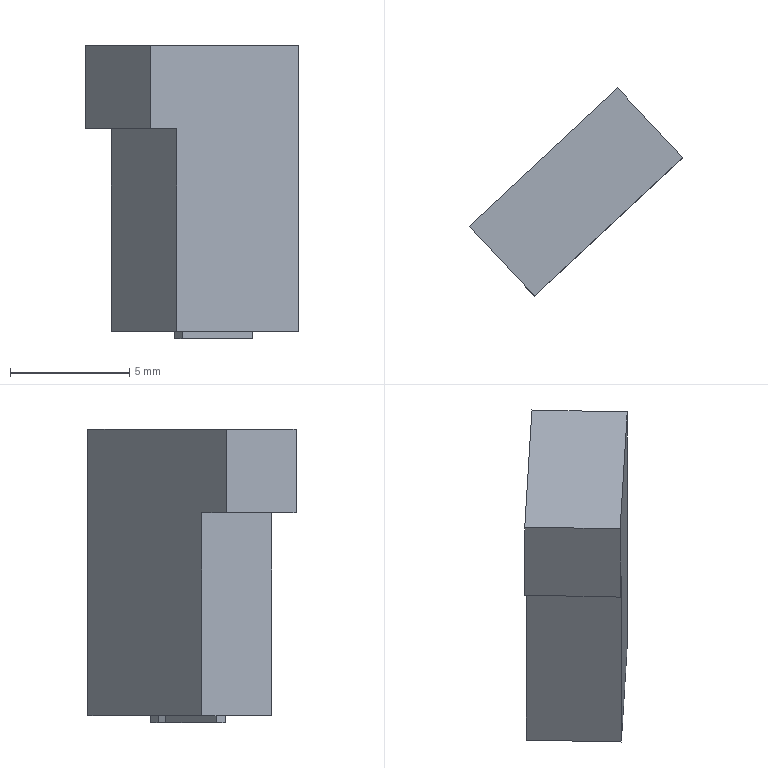Part | STEP file | gslz 2016.10.28-13_id950_x_t | 1 solid | 16 faces | box 8.945 x 8.722 x 12.3 mm | volume 357.729 mm3 | plane 15 | cylinder 1 | commonest cylinder face diameters 5.012 x1
STEP:
#1=CARTESIAN_POINT('',(0.,0.,0.));
#2=DIRECTION('',(0.,0.,1.));
#3=DIRECTION('',(1.,0.,0.));
#4=AXIS2_PLACEMENT_3D('',#1,#2,#3);
#5=CARTESIAN_POINT('',(-462.885,146.364,1.25));
#6=VERTEX_POINT('',#5);
#7=CARTESIAN_POINT('',(-462.538,146.688,1.25));
#8=VERTEX_POINT('',#7);
#9=CARTESIAN_POINT('',(-462.885,146.364,1.25));
#10=DIRECTION('',(0.7314,0.682,0.));
#11=VECTOR('',#10,1.);
#12=LINE('',#9,#11);
#13=CARTESIAN_POINT('',(-464.11,157.886,1.25));
#14=DIRECTION('',(0.,0.,-1.));
#15=DIRECTION('',(0.7314,0.682,0.));
#16=AXIS2_PLACEMENT_3D('',#13,#14,#15);
#17=PLANE('',#16);
#18=CARTESIAN_POINT('',(-6.962,9.262));
#19=DIRECTION('',(1.,0.));
#20=VECTOR('',#19,1.);
#21=LINE('',#18,#20);
#22=(GEOMETRIC_REPRESENTATION_CONTEXT(2)PARAMETRIC_REPRESENTATION_CONTEXT()REPRESENTATION_CONTEXT('',''));
#23=DEFINITIONAL_REPRESENTATION('',(#21),#22);
#24=PCURVE('',#17,#23);
#25=CARTESIAN_POINT('',(-462.885,146.364,0.95));
#26=DIRECTION('',(0.682,-0.7314,0.));
#27=DIRECTION('',(0.,0.,-1.));
#28=AXIS2_PLACEMENT_3D('',#25,#26,#27);
#29=PLANE('',#28);
#30=CARTESIAN_POINT('',(-0.3,0.));
#31=DIRECTION('',(0.,1.));
#32=VECTOR('',#31,1.);
#33=LINE('',#30,#32);
#34=(GEOMETRIC_REPRESENTATION_CONTEXT(2)PARAMETRIC_REPRESENTATION_CONTEXT()REPRESENTATION_CONTEXT('',''));
#35=DEFINITIONAL_REPRESENTATION('',(#33),#34);
#36=PCURVE('',#29,#35);
#37=SURFACE_CURVE('',#12,(#24,#36),.PCURVE_S1.);
#38=EDGE_CURVE('',#6,#8,#37,.T.);
#39=ORIENTED_EDGE('',*,*,#38,.F.);
#40=CARTESIAN_POINT('',(-461.783,146.049,1.25));
#41=VERTEX_POINT('',#40);
#42=CARTESIAN_POINT('',(-461.783,146.049,1.25));
#43=DIRECTION('',(-0.9615,0.2748,0.));
#44=VECTOR('',#43,1.);
#45=LINE('',#42,#44);
#46=CARTESIAN_POINT('',(-6.371,10.245));
#47=DIRECTION('',(-0.5158,-0.8567));
#48=VECTOR('',#47,1.);
#49=LINE('',#46,#48);
#50=(GEOMETRIC_REPRESENTATION_CONTEXT(2)PARAMETRIC_REPRESENTATION_CONTEXT()REPRESENTATION_CONTEXT('',''));
#51=DEFINITIONAL_REPRESENTATION('',(#49),#50);
#52=PCURVE('',#17,#51);
#53=CARTESIAN_POINT('',(-461.783,146.049,0.95));
#54=DIRECTION('',(0.2748,0.9615,0.));
#55=DIRECTION('',(-0.9615,0.2748,0.));
#56=AXIS2_PLACEMENT_3D('',#53,#54,#55);
#57=PLANE('',#56);
#58=CARTESIAN_POINT('',(0.,0.3));
#59=DIRECTION('',(1.,0.));
#60=VECTOR('',#59,1.);
#61=LINE('',#58,#60);
#62=(GEOMETRIC_REPRESENTATION_CONTEXT(2)PARAMETRIC_REPRESENTATION_CONTEXT()REPRESENTATION_CONTEXT('',''));
#63=DEFINITIONAL_REPRESENTATION('',(#61),#62);
#64=PCURVE('',#57,#63);
#65=SURFACE_CURVE('',#45,(#52,#64),.PCURVE_S1.);
#66=EDGE_CURVE('',#41,#6,#65,.T.);
#67=ORIENTED_EDGE('',*,*,#66,.F.);
#68=CARTESIAN_POINT('',(-464.072,143.915,1.25));
#69=VERTEX_POINT('',#68);
#70=CARTESIAN_POINT('',(-464.072,143.915,1.25));
#71=DIRECTION('',(0.7314,0.682,0.));
#72=VECTOR('',#71,1.);
#73=LINE('',#70,#72);
#74=CARTESIAN_POINT('',(-9.5,10.245));
#75=DIRECTION('',(1.,0.));
#76=VECTOR('',#75,1.);
#77=LINE('',#74,#76);
#78=(GEOMETRIC_REPRESENTATION_CONTEXT(2)PARAMETRIC_REPRESENTATION_CONTEXT()REPRESENTATION_CONTEXT('',''));
#79=DEFINITIONAL_REPRESENTATION('',(#77),#78);
#80=PCURVE('',#17,#79);
#81=CARTESIAN_POINT('',(-464.072,143.915,0.95));
#82=DIRECTION('',(0.682,-0.7314,0.));
#83=DIRECTION('',(0.,0.,-1.));
#84=AXIS2_PLACEMENT_3D('',#81,#82,#83);
#85=PLANE('',#84);
#86=CARTESIAN_POINT('',(-0.3,0.));
#87=DIRECTION('',(0.,1.));
#88=VECTOR('',#87,1.);
#89=LINE('',#86,#88);
#90=(GEOMETRIC_REPRESENTATION_CONTEXT(2)PARAMETRIC_REPRESENTATION_CONTEXT()REPRESENTATION_CONTEXT('',''));
#91=DEFINITIONAL_REPRESENTATION('',(#89),#90);
#92=PCURVE('',#85,#91);
#93=SURFACE_CURVE('',#73,(#80,#92),.PCURVE_S1.);
#94=EDGE_CURVE('',#69,#41,#93,.T.);
#95=ORIENTED_EDGE('',*,*,#94,.F.);
#96=CARTESIAN_POINT('',(-463.737,143.555,1.25));
#97=VERTEX_POINT('',#96);
#98=CARTESIAN_POINT('',(-463.737,143.555,1.25));
#99=DIRECTION('',(-0.682,0.7314,0.));
#100=VECTOR('',#99,1.);
#101=LINE('',#98,#100);
#102=CARTESIAN_POINT('',(-9.5,10.736));
#103=DIRECTION('',(0.,-1.));
#104=VECTOR('',#103,1.);
#105=LINE('',#102,#104);
#106=(GEOMETRIC_REPRESENTATION_CONTEXT(2)PARAMETRIC_REPRESENTATION_CONTEXT()REPRESENTATION_CONTEXT('',''));
#107=DEFINITIONAL_REPRESENTATION('',(#105),#106);
#108=PCURVE('',#17,#107);
#109=CARTESIAN_POINT('',(-463.737,143.555,0.95));
#110=DIRECTION('',(0.7314,0.682,0.));
#111=DIRECTION('',(0.,0.,1.));
#112=AXIS2_PLACEMENT_3D('',#109,#110,#111);
#113=PLANE('',#112);
#114=CARTESIAN_POINT('',(0.3,0.));
#115=DIRECTION('',(0.,-1.));
#116=VECTOR('',#115,1.);
#117=LINE('',#114,#116);
#118=(GEOMETRIC_REPRESENTATION_CONTEXT(2)PARAMETRIC_REPRESENTATION_CONTEXT()REPRESENTATION_CONTEXT('',''));
#119=DEFINITIONAL_REPRESENTATION('',(#117),#118);
#120=PCURVE('',#113,#119);
#121=SURFACE_CURVE('',#101,(#108,#120),.PCURVE_S1.);
#122=EDGE_CURVE('',#97,#69,#121,.T.);
#123=ORIENTED_EDGE('',*,*,#122,.F.);
#124=CARTESIAN_POINT('',(-460.799,146.295,1.25));
#125=VERTEX_POINT('',#124);
#126=CARTESIAN_POINT('',(-460.799,146.295,1.25));
#127=DIRECTION('',(-0.7314,-0.682,0.));
#128=VECTOR('',#127,1.);
#129=LINE('',#126,#128);
#130=CARTESIAN_POINT('',(-5.484,10.736));
#131=DIRECTION('',(-1.,0.));
#132=VECTOR('',#131,1.);
#133=LINE('',#130,#132);
#134=(GEOMETRIC_REPRESENTATION_CONTEXT(2)PARAMETRIC_REPRESENTATION_CONTEXT()REPRESENTATION_CONTEXT('',''));
#135=DEFINITIONAL_REPRESENTATION('',(#133),#134);
#136=PCURVE('',#17,#135);
#137=CARTESIAN_POINT('',(-460.799,146.295,0.95));
#138=DIRECTION('',(-0.682,0.7314,0.));
#139=DIRECTION('',(0.,0.,1.));
#140=AXIS2_PLACEMENT_3D('',#137,#138,#139);
#141=PLANE('',#140);
#142=CARTESIAN_POINT('',(0.3,0.));
#143=DIRECTION('',(0.,-1.));
#144=VECTOR('',#143,1.);
#145=LINE('',#142,#144);
#146=(GEOMETRIC_REPRESENTATION_CONTEXT(2)PARAMETRIC_REPRESENTATION_CONTEXT()REPRESENTATION_CONTEXT('',''));
#147=DEFINITIONAL_REPRESENTATION('',(#145),#146);
#148=PCURVE('',#141,#147);
#149=SURFACE_CURVE('',#129,(#136,#148),.PCURVE_S1.);
#150=EDGE_CURVE('',#125,#97,#149,.T.);
#151=ORIENTED_EDGE('',*,*,#150,.F.);
#152=CARTESIAN_POINT('',(-461.015,146.527,1.25));
#153=VERTEX_POINT('',#152);
#154=CARTESIAN_POINT('',(-461.015,146.527,1.25));
#155=DIRECTION('',(0.682,-0.7314,0.));
#156=VECTOR('',#155,1.);
#157=LINE('',#154,#156);
#158=CARTESIAN_POINT('',(-5.484,10.419));
#159=DIRECTION('',(0.,1.));
#160=VECTOR('',#159,1.);
#161=LINE('',#158,#160);
#162=(GEOMETRIC_REPRESENTATION_CONTEXT(2)PARAMETRIC_REPRESENTATION_CONTEXT()REPRESENTATION_CONTEXT('',''));
#163=DEFINITIONAL_REPRESENTATION('',(#161),#162);
#164=PCURVE('',#17,#163);
#165=CARTESIAN_POINT('',(-461.015,146.527,0.95));
#166=DIRECTION('',(-0.7314,-0.682,0.));
#167=DIRECTION('',(0.,0.,-1.));
#168=AXIS2_PLACEMENT_3D('',#165,#166,#167);
#169=PLANE('',#168);
#170=CARTESIAN_POINT('',(-0.3,0.));
#171=DIRECTION('',(0.,1.));
#172=VECTOR('',#171,1.);
#173=LINE('',#170,#172);
#174=(GEOMETRIC_REPRESENTATION_CONTEXT(2)PARAMETRIC_REPRESENTATION_CONTEXT()REPRESENTATION_CONTEXT('',''));
#175=DEFINITIONAL_REPRESENTATION('',(#173),#174);
#176=PCURVE('',#169,#175);
#177=SURFACE_CURVE('',#157,(#164,#176),.PCURVE_S1.);
#178=EDGE_CURVE('',#153,#125,#177,.T.);
#179=ORIENTED_EDGE('',*,*,#178,.F.);
#180=CARTESIAN_POINT('',(-461.526,148.98,1.25));
#181=DIRECTION('',(0.,0.,1.));
#182=DIRECTION('',(0.682,-0.7314,0.));
#183=AXIS2_PLACEMENT_3D('',#180,#181,#182);
#184=CIRCLE('',#183,2.506);
#185=CARTESIAN_POINT('',(-4.184,10.782));
#186=CARTESIAN_POINT('',(0.1568,10.782));
#187=CARTESIAN_POINT('',(-2.013,7.023));
#188=CARTESIAN_POINT('',(-4.184,3.264));
#189=CARTESIAN_POINT('',(-6.354,7.023));
#190=CARTESIAN_POINT('',(-8.524,10.782));
#191=CARTESIAN_POINT('',(-4.184,10.782));
#192=(BOUNDED_CURVE()B_SPLINE_CURVE(2,(#185,#186,#187,#188,#189,#190,#191),.UNSPECIFIED.,.T.,.F.)B_SPLINE_CURVE_WITH_KNOTS((1,2,2,2,2,1),(-2.094,0.,2.094,4.189,6.283,8.378),.UNSPECIFIED.)CURVE()GEOMETRIC_REPRESENTATION_ITEM()RATIONAL_B_SPLINE_CURVE((1.,0.5,1.,0.5,1.,0.5,1.))REPRESENTATION_ITEM(''));
#193=(GEOMETRIC_REPRESENTATION_CONTEXT(2)PARAMETRIC_REPRESENTATION_CONTEXT()REPRESENTATION_CONTEXT('',''));
#194=DEFINITIONAL_REPRESENTATION('',(#192),#193);
#195=PCURVE('',#17,#194);
#196=CARTESIAN_POINT('',(-461.526,148.98,0.95));
#197=DIRECTION('',(0.,0.,1.));
#198=DIRECTION('',(0.682,-0.7314,0.));
#199=AXIS2_PLACEMENT_3D('',#196,#197,#198);
#200=CYLINDRICAL_SURFACE('',#199,2.506);
#201=CARTESIAN_POINT('',(0.,0.3));
#202=DIRECTION('',(1.,0.));
#203=VECTOR('',#202,1.);
#204=LINE('',#201,#203);
#205=(GEOMETRIC_REPRESENTATION_CONTEXT(2)PARAMETRIC_REPRESENTATION_CONTEXT()REPRESENTATION_CONTEXT('',''));
#206=DEFINITIONAL_REPRESENTATION('',(#204),#205);
#207=PCURVE('',#200,#206);
#208=SURFACE_CURVE('',#184,(#195,#207),.PCURVE_S1.);
#209=EDGE_CURVE('',#8,#153,#208,.T.);
#210=ORIENTED_EDGE('',*,*,#209,.F.);
#211=EDGE_LOOP('',(#39,#67,#95,#123,#151,#179,#210));
#212=FACE_BOUND('',#211,.T.);
#213=CARTESIAN_POINT('',(-466.7,144.534,1.25));
#214=VERTEX_POINT('',#213);
#215=CARTESIAN_POINT('',(-461.58,149.308,1.25));
#216=VERTEX_POINT('',#215);
#217=CARTESIAN_POINT('',(-466.7,144.534,1.25));
#218=DIRECTION('',(0.7314,0.682,0.));
#219=VECTOR('',#218,1.);
#220=LINE('',#217,#219);
#221=CARTESIAN_POINT('',(-11.,7.999));
#222=DIRECTION('',(1.,0.));
#223=VECTOR('',#222,1.);
#224=LINE('',#221,#223);
#225=(GEOMETRIC_REPRESENTATION_CONTEXT(2)PARAMETRIC_REPRESENTATION_CONTEXT()REPRESENTATION_CONTEXT('',''));
#226=DEFINITIONAL_REPRESENTATION('',(#224),#225);
#227=PCURVE('',#17,#226);
#228=CARTESIAN_POINT('',(-466.7,144.534,-0.75));
#229=DIRECTION('',(0.682,-0.7314,0.));
#230=DIRECTION('',(0.,0.,-1.));
#231=AXIS2_PLACEMENT_3D('',#228,#229,#230);
#232=PLANE('',#231);
#233=CARTESIAN_POINT('',(-2.,0.));
#234=DIRECTION('',(0.,1.));
#235=VECTOR('',#234,1.);
#236=LINE('',#233,#235);
#237=(GEOMETRIC_REPRESENTATION_CONTEXT(2)PARAMETRIC_REPRESENTATION_CONTEXT()REPRESENTATION_CONTEXT('',''));
#238=DEFINITIONAL_REPRESENTATION('',(#236),#237);
#239=PCURVE('',#232,#238);
#240=SURFACE_CURVE('',#220,(#227,#239),.PCURVE_S1.);
#241=EDGE_CURVE('',#214,#216,#240,.T.);
#242=ORIENTED_EDGE('',*,*,#241,.T.);
#243=CARTESIAN_POINT('',(-458.853,146.382,1.25));
#244=VERTEX_POINT('',#243);
#245=CARTESIAN_POINT('',(-461.58,149.308,1.25));
#246=DIRECTION('',(0.682,-0.7314,0.));
#247=VECTOR('',#246,1.);
#248=LINE('',#245,#247);
#249=CARTESIAN_POINT('',(-4.,7.999));
#250=DIRECTION('',(0.,1.));
#251=VECTOR('',#250,1.);
#252=LINE('',#249,#251);
#253=(GEOMETRIC_REPRESENTATION_CONTEXT(2)PARAMETRIC_REPRESENTATION_CONTEXT()REPRESENTATION_CONTEXT('',''));
#254=DEFINITIONAL_REPRESENTATION('',(#252),#253);
#255=PCURVE('',#17,#254);
#256=CARTESIAN_POINT('',(-461.58,149.308,-0.75));
#257=DIRECTION('',(-0.7314,-0.682,0.));
#258=DIRECTION('',(0.,0.,-1.));
#259=AXIS2_PLACEMENT_3D('',#256,#257,#258);
#260=PLANE('',#259);
#261=CARTESIAN_POINT('',(-2.,0.));
#262=DIRECTION('',(0.,1.));
#263=VECTOR('',#262,1.);
#264=LINE('',#261,#263);
#265=(GEOMETRIC_REPRESENTATION_CONTEXT(2)PARAMETRIC_REPRESENTATION_CONTEXT()REPRESENTATION_CONTEXT('',''));
#266=DEFINITIONAL_REPRESENTATION('',(#264),#265);
#267=PCURVE('',#260,#266);
#268=SURFACE_CURVE('',#248,(#255,#267),.PCURVE_S1.);
#269=EDGE_CURVE('',#216,#244,#268,.T.);
#270=ORIENTED_EDGE('',*,*,#269,.T.);
#271=CARTESIAN_POINT('',(-463.972,141.609,1.25));
#272=VERTEX_POINT('',#271);
#273=CARTESIAN_POINT('',(-458.853,146.382,1.25));
#274=DIRECTION('',(-0.7314,-0.682,0.));
#275=VECTOR('',#274,1.);
#276=LINE('',#273,#275);
#277=CARTESIAN_POINT('',(-4.,11.999));
#278=DIRECTION('',(-1.,0.));
#279=VECTOR('',#278,1.);
#280=LINE('',#277,#279);
#281=(GEOMETRIC_REPRESENTATION_CONTEXT(2)PARAMETRIC_REPRESENTATION_CONTEXT()REPRESENTATION_CONTEXT('',''));
#282=DEFINITIONAL_REPRESENTATION('',(#280),#281);
#283=PCURVE('',#17,#282);
#284=CARTESIAN_POINT('',(-458.853,146.382,-0.75));
#285=DIRECTION('',(-0.682,0.7314,0.));
#286=DIRECTION('',(0.,0.,1.));
#287=AXIS2_PLACEMENT_3D('',#284,#285,#286);
#288=PLANE('',#287);
#289=CARTESIAN_POINT('',(2.,0.));
#290=DIRECTION('',(0.,-1.));
#291=VECTOR('',#290,1.);
#292=LINE('',#289,#291);
#293=(GEOMETRIC_REPRESENTATION_CONTEXT(2)PARAMETRIC_REPRESENTATION_CONTEXT()REPRESENTATION_CONTEXT('',''));
#294=DEFINITIONAL_REPRESENTATION('',(#292),#293);
#295=PCURVE('',#288,#294);
#296=SURFACE_CURVE('',#276,(#283,#295),.PCURVE_S1.);
#297=EDGE_CURVE('',#244,#272,#296,.T.);
#298=ORIENTED_EDGE('',*,*,#297,.T.);
#299=CARTESIAN_POINT('',(-463.972,141.609,1.25));
#300=DIRECTION('',(-0.682,0.7314,0.));
#301=VECTOR('',#300,1.);
#302=LINE('',#299,#301);
#303=CARTESIAN_POINT('',(-11.,11.999));
#304=DIRECTION('',(0.,-1.));
#305=VECTOR('',#304,1.);
#306=LINE('',#303,#305);
#307=(GEOMETRIC_REPRESENTATION_CONTEXT(2)PARAMETRIC_REPRESENTATION_CONTEXT()REPRESENTATION_CONTEXT('',''));
#308=DEFINITIONAL_REPRESENTATION('',(#306),#307);
#309=PCURVE('',#17,#308);
#310=CARTESIAN_POINT('',(-463.972,141.609,-0.75));
#311=DIRECTION('',(0.7314,0.682,0.));
#312=DIRECTION('',(0.,0.,1.));
#313=AXIS2_PLACEMENT_3D('',#310,#311,#312);
#314=PLANE('',#313);
#315=CARTESIAN_POINT('',(2.,0.));
#316=DIRECTION('',(0.,-1.));
#317=VECTOR('',#316,1.);
#318=LINE('',#315,#317);
#319=(GEOMETRIC_REPRESENTATION_CONTEXT(2)PARAMETRIC_REPRESENTATION_CONTEXT()REPRESENTATION_CONTEXT('',''));
#320=DEFINITIONAL_REPRESENTATION('',(#318),#319);
#321=PCURVE('',#314,#320);
#322=SURFACE_CURVE('',#302,(#309,#321),.PCURVE_S1.);
#323=EDGE_CURVE('',#272,#214,#322,.T.);
#324=ORIENTED_EDGE('',*,*,#323,.T.);
#325=EDGE_LOOP('',(#242,#270,#298,#324));
#326=FACE_BOUND('',#325,.T.);
#327=ADVANCED_FACE('',(#212,#326),#17,.T.);
#328=CARTESIAN_POINT('',(-467.797,143.511,13.25));
#329=VERTEX_POINT('',#328);
#330=CARTESIAN_POINT('',(-461.58,149.308,13.25));
#331=VERTEX_POINT('',#330);
#332=CARTESIAN_POINT('',(-466.7,144.534,13.25));
#333=DIRECTION('',(0.7314,0.682,0.));
#334=VECTOR('',#333,1.);
#335=LINE('',#332,#334);
#336=CARTESIAN_POINT('',(-14.,0.));
#337=DIRECTION('',(0.,1.));
#338=VECTOR('',#337,1.);
#339=LINE('',#336,#338);
#340=(GEOMETRIC_REPRESENTATION_CONTEXT(2)PARAMETRIC_REPRESENTATION_CONTEXT()REPRESENTATION_CONTEXT('',''));
#341=DEFINITIONAL_REPRESENTATION('',(#339),#340);
#342=PCURVE('',#232,#341);
#343=CARTESIAN_POINT('',(-464.11,157.886,13.25));
#344=DIRECTION('',(0.,0.,-1.));
#345=DIRECTION('',(0.7314,0.682,0.));
#346=AXIS2_PLACEMENT_3D('',#343,#344,#345);
#347=PLANE('',#346);
#348=CARTESIAN_POINT('',(-11.,7.999));
#349=DIRECTION('',(1.,0.));
#350=VECTOR('',#349,1.);
#351=LINE('',#348,#350);
#352=(GEOMETRIC_REPRESENTATION_CONTEXT(2)PARAMETRIC_REPRESENTATION_CONTEXT()REPRESENTATION_CONTEXT('',''));
#353=DEFINITIONAL_REPRESENTATION('',(#351),#352);
#354=PCURVE('',#347,#353);
#355=SURFACE_CURVE('',#335,(#342,#354),.PCURVE_S1.);
#356=EDGE_CURVE('',#329,#331,#355,.T.);
#357=ORIENTED_EDGE('',*,*,#356,.T.);
#358=CARTESIAN_POINT('',(-461.58,149.308,-0.75));
#359=DIRECTION('',(0.,0.,1.));
#360=VECTOR('',#359,1.);
#361=LINE('',#358,#360);
#362=CARTESIAN_POINT('',(0.,7.));
#363=DIRECTION('',(-1.,0.));
#364=VECTOR('',#363,1.);
#365=LINE('',#362,#364);
#366=(GEOMETRIC_REPRESENTATION_CONTEXT(2)PARAMETRIC_REPRESENTATION_CONTEXT()REPRESENTATION_CONTEXT('',''));
#367=DEFINITIONAL_REPRESENTATION('',(#365),#366);
#368=PCURVE('',#232,#367);
#369=CARTESIAN_POINT('',(0.,0.));
#370=DIRECTION('',(-1.,0.));
#371=VECTOR('',#370,1.);
#372=LINE('',#369,#371);
#373=(GEOMETRIC_REPRESENTATION_CONTEXT(2)PARAMETRIC_REPRESENTATION_CONTEXT()REPRESENTATION_CONTEXT('',''));
#374=DEFINITIONAL_REPRESENTATION('',(#372),#373);
#375=PCURVE('',#260,#374);
#376=SURFACE_CURVE('',#361,(#368,#375),.PCURVE_S1.);
#377=EDGE_CURVE('',#216,#331,#376,.T.);
#378=ORIENTED_EDGE('',*,*,#377,.F.);
#379=ORIENTED_EDGE('',*,*,#241,.F.);
#380=CARTESIAN_POINT('',(-466.7,144.534,9.75));
#381=VERTEX_POINT('',#380);
#382=CARTESIAN_POINT('',(-466.7,144.534,-0.75));
#383=DIRECTION('',(0.,0.,1.));
#384=VECTOR('',#383,1.);
#385=LINE('',#382,#384);
#386=CARTESIAN_POINT('',(0.,0.));
#387=DIRECTION('',(-1.,0.));
#388=VECTOR('',#387,1.);
#389=LINE('',#386,#388);
#390=(GEOMETRIC_REPRESENTATION_CONTEXT(2)PARAMETRIC_REPRESENTATION_CONTEXT()REPRESENTATION_CONTEXT('',''));
#391=DEFINITIONAL_REPRESENTATION('',(#389),#390);
#392=PCURVE('',#232,#391);
#393=CARTESIAN_POINT('',(0.,-4.));
#394=DIRECTION('',(1.,0.));
#395=VECTOR('',#394,1.);
#396=LINE('',#393,#395);
#397=(GEOMETRIC_REPRESENTATION_CONTEXT(2)PARAMETRIC_REPRESENTATION_CONTEXT()REPRESENTATION_CONTEXT('',''));
#398=DEFINITIONAL_REPRESENTATION('',(#396),#397);
#399=PCURVE('',#314,#398);
#400=SURFACE_CURVE('',#385,(#392,#399),.PCURVE_S1.);
#401=EDGE_CURVE('',#214,#381,#400,.T.);
#402=ORIENTED_EDGE('',*,*,#401,.T.);
#403=CARTESIAN_POINT('',(-467.797,143.511,9.75));
#404=VERTEX_POINT('',#403);
#405=CARTESIAN_POINT('',(-467.797,143.511,9.75));
#406=DIRECTION('',(0.7314,0.682,0.));
#407=VECTOR('',#406,1.);
#408=LINE('',#405,#407);
#409=CARTESIAN_POINT('',(-10.5,-1.5));
#410=DIRECTION('',(0.,1.));
#411=VECTOR('',#410,1.);
#412=LINE('',#409,#411);
#413=(GEOMETRIC_REPRESENTATION_CONTEXT(2)PARAMETRIC_REPRESENTATION_CONTEXT()REPRESENTATION_CONTEXT('',''));
#414=DEFINITIONAL_REPRESENTATION('',(#412),#413);
#415=PCURVE('',#232,#414);
#416=CARTESIAN_POINT('',(-465.069,140.586,9.75));
#417=DIRECTION('',(0.,0.,-1.));
#418=DIRECTION('',(0.7314,0.682,0.));
#419=AXIS2_PLACEMENT_3D('',#416,#417,#418);
#420=PLANE('',#419);
#421=CARTESIAN_POINT('',(0.,-4.));
#422=DIRECTION('',(1.,0.));
#423=VECTOR('',#422,1.);
#424=LINE('',#421,#423);
#425=(GEOMETRIC_REPRESENTATION_CONTEXT(2)PARAMETRIC_REPRESENTATION_CONTEXT()REPRESENTATION_CONTEXT('',''));
#426=DEFINITIONAL_REPRESENTATION('',(#424),#425);
#427=PCURVE('',#420,#426);
#428=SURFACE_CURVE('',#408,(#415,#427),.PCURVE_S1.);
#429=EDGE_CURVE('',#404,#381,#428,.T.);
#430=ORIENTED_EDGE('',*,*,#429,.F.);
#431=CARTESIAN_POINT('',(-467.797,143.511,13.25));
#432=DIRECTION('',(0.,0.,-1.));
#433=VECTOR('',#432,1.);
#434=LINE('',#431,#433);
#435=CARTESIAN_POINT('',(-14.,-1.5));
#436=DIRECTION('',(1.,0.));
#437=VECTOR('',#436,1.);
#438=LINE('',#435,#437);
#439=(GEOMETRIC_REPRESENTATION_CONTEXT(2)PARAMETRIC_REPRESENTATION_CONTEXT()REPRESENTATION_CONTEXT('',''));
#440=DEFINITIONAL_REPRESENTATION('',(#438),#439);
#441=PCURVE('',#232,#440);
#442=CARTESIAN_POINT('',(-465.069,140.586,13.25));
#443=DIRECTION('',(-0.7314,-0.682,0.));
#444=DIRECTION('',(-0.682,0.7314,0.));
#445=AXIS2_PLACEMENT_3D('',#442,#443,#444);
#446=PLANE('',#445);
#447=CARTESIAN_POINT('',(4.,0.));
#448=DIRECTION('',(0.,1.));
#449=VECTOR('',#448,1.);
#450=LINE('',#447,#449);
#451=(GEOMETRIC_REPRESENTATION_CONTEXT(2)PARAMETRIC_REPRESENTATION_CONTEXT()REPRESENTATION_CONTEXT('',''));
#452=DEFINITIONAL_REPRESENTATION('',(#450),#451);
#453=PCURVE('',#446,#452);
#454=SURFACE_CURVE('',#434,(#441,#453),.PCURVE_S1.);
#455=EDGE_CURVE('',#329,#404,#454,.T.);
#456=ORIENTED_EDGE('',*,*,#455,.F.);
#457=EDGE_LOOP('',(#357,#378,#379,#402,#430,#456));
#458=FACE_BOUND('',#457,.T.);
#459=ADVANCED_FACE('',(#458),#232,.F.);
#460=CARTESIAN_POINT('',(-458.853,146.382,13.25));
#461=VERTEX_POINT('',#460);
#462=CARTESIAN_POINT('',(-461.58,149.308,13.25));
#463=DIRECTION('',(0.682,-0.7314,0.));
#464=VECTOR('',#463,1.);
#465=LINE('',#462,#464);
#466=CARTESIAN_POINT('',(-14.,0.));
#467=DIRECTION('',(0.,1.));
#468=VECTOR('',#467,1.);
#469=LINE('',#466,#468);
#470=(GEOMETRIC_REPRESENTATION_CONTEXT(2)PARAMETRIC_REPRESENTATION_CONTEXT()REPRESENTATION_CONTEXT('',''));
#471=DEFINITIONAL_REPRESENTATION('',(#469),#470);
#472=PCURVE('',#260,#471);
#473=CARTESIAN_POINT('',(-4.,7.999));
#474=DIRECTION('',(0.,1.));
#475=VECTOR('',#474,1.);
#476=LINE('',#473,#475);
#477=(GEOMETRIC_REPRESENTATION_CONTEXT(2)PARAMETRIC_REPRESENTATION_CONTEXT()REPRESENTATION_CONTEXT('',''));
#478=DEFINITIONAL_REPRESENTATION('',(#476),#477);
#479=PCURVE('',#347,#478);
#480=SURFACE_CURVE('',#465,(#472,#479),.PCURVE_S1.);
#481=EDGE_CURVE('',#331,#461,#480,.T.);
#482=ORIENTED_EDGE('',*,*,#481,.T.);
#483=CARTESIAN_POINT('',(-458.853,146.382,-0.75));
#484=DIRECTION('',(0.,0.,1.));
#485=VECTOR('',#484,1.);
#486=LINE('',#483,#485);
#487=CARTESIAN_POINT('',(0.,4.));
#488=DIRECTION('',(-1.,0.));
#489=VECTOR('',#488,1.);
#490=LINE('',#487,#489);
#491=(GEOMETRIC_REPRESENTATION_CONTEXT(2)PARAMETRIC_REPRESENTATION_CONTEXT()REPRESENTATION_CONTEXT('',''));
#492=DEFINITIONAL_REPRESENTATION('',(#490),#491);
#493=PCURVE('',#260,#492);
#494=CARTESIAN_POINT('',(0.,0.));
#495=DIRECTION('',(1.,0.));
#496=VECTOR('',#495,1.);
#497=LINE('',#494,#496);
#498=(GEOMETRIC_REPRESENTATION_CONTEXT(2)PARAMETRIC_REPRESENTATION_CONTEXT()REPRESENTATION_CONTEXT('',''));
#499=DEFINITIONAL_REPRESENTATION('',(#497),#498);
#500=PCURVE('',#288,#499);
#501=SURFACE_CURVE('',#486,(#493,#500),.PCURVE_S1.);
#502=EDGE_CURVE('',#244,#461,#501,.T.);
#503=ORIENTED_EDGE('',*,*,#502,.F.);
#504=ORIENTED_EDGE('',*,*,#269,.F.);
#505=ORIENTED_EDGE('',*,*,#377,.T.);
#506=EDGE_LOOP('',(#482,#503,#504,#505));
#507=FACE_BOUND('',#506,.T.);
#508=ADVANCED_FACE('',(#507),#260,.F.);
#509=CARTESIAN_POINT('',(-465.069,140.586,13.25));
#510=VERTEX_POINT('',#509);
#511=CARTESIAN_POINT('',(-458.853,146.382,13.25));
#512=DIRECTION('',(-0.7314,-0.682,0.));
#513=VECTOR('',#512,1.);
#514=LINE('',#511,#513);
#515=CARTESIAN_POINT('',(14.,0.));
#516=DIRECTION('',(0.,-1.));
#517=VECTOR('',#516,1.);
#518=LINE('',#515,#517);
#519=(GEOMETRIC_REPRESENTATION_CONTEXT(2)PARAMETRIC_REPRESENTATION_CONTEXT()REPRESENTATION_CONTEXT('',''));
#520=DEFINITIONAL_REPRESENTATION('',(#518),#519);
#521=PCURVE('',#288,#520);
#522=CARTESIAN_POINT('',(-4.,11.999));
#523=DIRECTION('',(-1.,0.));
#524=VECTOR('',#523,1.);
#525=LINE('',#522,#524);
#526=(GEOMETRIC_REPRESENTATION_CONTEXT(2)PARAMETRIC_REPRESENTATION_CONTEXT()REPRESENTATION_CONTEXT('',''));
#527=DEFINITIONAL_REPRESENTATION('',(#525),#526);
#528=PCURVE('',#347,#527);
#529=SURFACE_CURVE('',#514,(#521,#528),.PCURVE_S1.);
#530=EDGE_CURVE('',#461,#510,#529,.T.);
#531=ORIENTED_EDGE('',*,*,#530,.T.);
#532=CARTESIAN_POINT('',(-465.069,140.586,9.75));
#533=VERTEX_POINT('',#532);
#534=CARTESIAN_POINT('',(-465.069,140.586,13.25));
#535=DIRECTION('',(0.,0.,-1.));
#536=VECTOR('',#535,1.);
#537=LINE('',#534,#536);
#538=CARTESIAN_POINT('',(14.,-8.5));
#539=DIRECTION('',(-1.,0.));
#540=VECTOR('',#539,1.);
#541=LINE('',#538,#540);
#542=(GEOMETRIC_REPRESENTATION_CONTEXT(2)PARAMETRIC_REPRESENTATION_CONTEXT()REPRESENTATION_CONTEXT('',''));
#543=DEFINITIONAL_REPRESENTATION('',(#541),#542);
#544=PCURVE('',#288,#543);
#545=CARTESIAN_POINT('',(0.,0.));
#546=DIRECTION('',(0.,1.));
#547=VECTOR('',#546,1.);
#548=LINE('',#545,#547);
#549=(GEOMETRIC_REPRESENTATION_CONTEXT(2)PARAMETRIC_REPRESENTATION_CONTEXT()REPRESENTATION_CONTEXT('',''));
#550=DEFINITIONAL_REPRESENTATION('',(#548),#549);
#551=PCURVE('',#446,#550);
#552=SURFACE_CURVE('',#537,(#544,#551),.PCURVE_S1.);
#553=EDGE_CURVE('',#510,#533,#552,.T.);
#554=ORIENTED_EDGE('',*,*,#553,.T.);
#555=CARTESIAN_POINT('',(-463.972,141.609,9.75));
#556=VERTEX_POINT('',#555);
#557=CARTESIAN_POINT('',(-465.069,140.586,9.75));
#558=DIRECTION('',(0.7314,0.682,0.));
#559=VECTOR('',#558,1.);
#560=LINE('',#557,#559);
#561=CARTESIAN_POINT('',(10.5,-8.5));
#562=DIRECTION('',(0.,1.));
#563=VECTOR('',#562,1.);
#564=LINE('',#561,#563);
#565=(GEOMETRIC_REPRESENTATION_CONTEXT(2)PARAMETRIC_REPRESENTATION_CONTEXT()REPRESENTATION_CONTEXT('',''));
#566=DEFINITIONAL_REPRESENTATION('',(#564),#565);
#567=PCURVE('',#288,#566);
#568=CARTESIAN_POINT('',(0.,0.));
#569=DIRECTION('',(1.,0.));
#570=VECTOR('',#569,1.);
#571=LINE('',#568,#570);
#572=(GEOMETRIC_REPRESENTATION_CONTEXT(2)PARAMETRIC_REPRESENTATION_CONTEXT()REPRESENTATION_CONTEXT('',''));
#573=DEFINITIONAL_REPRESENTATION('',(#571),#572);
#574=PCURVE('',#420,#573);
#575=SURFACE_CURVE('',#560,(#567,#574),.PCURVE_S1.);
#576=EDGE_CURVE('',#533,#556,#575,.T.);
#577=ORIENTED_EDGE('',*,*,#576,.T.);
#578=CARTESIAN_POINT('',(-463.972,141.609,-0.75));
#579=DIRECTION('',(0.,0.,1.));
#580=VECTOR('',#579,1.);
#581=LINE('',#578,#580);
#582=CARTESIAN_POINT('',(0.,-7.));
#583=DIRECTION('',(1.,0.));
#584=VECTOR('',#583,1.);
#585=LINE('',#582,#584);
#586=(GEOMETRIC_REPRESENTATION_CONTEXT(2)PARAMETRIC_REPRESENTATION_CONTEXT()REPRESENTATION_CONTEXT('',''));
#587=DEFINITIONAL_REPRESENTATION('',(#585),#586);
#588=PCURVE('',#288,#587);
#589=CARTESIAN_POINT('',(0.,0.));
#590=DIRECTION('',(1.,0.));
#591=VECTOR('',#590,1.);
#592=LINE('',#589,#591);
#593=(GEOMETRIC_REPRESENTATION_CONTEXT(2)PARAMETRIC_REPRESENTATION_CONTEXT()REPRESENTATION_CONTEXT('',''));
#594=DEFINITIONAL_REPRESENTATION('',(#592),#593);
#595=PCURVE('',#314,#594);
#596=SURFACE_CURVE('',#581,(#588,#595),.PCURVE_S1.);
#597=EDGE_CURVE('',#272,#556,#596,.T.);
#598=ORIENTED_EDGE('',*,*,#597,.F.);
#599=ORIENTED_EDGE('',*,*,#297,.F.);
#600=ORIENTED_EDGE('',*,*,#502,.T.);
#601=EDGE_LOOP('',(#531,#554,#577,#598,#599,#600));
#602=FACE_BOUND('',#601,.T.);
#603=ADVANCED_FACE('',(#602),#288,.F.);
#604=ORIENTED_EDGE('',*,*,#597,.T.);
#605=CARTESIAN_POINT('',(-463.972,141.609,9.75));
#606=DIRECTION('',(-0.682,0.7314,0.));
#607=VECTOR('',#606,1.);
#608=LINE('',#605,#607);
#609=CARTESIAN_POINT('',(10.5,0.));
#610=DIRECTION('',(0.,-1.));
#611=VECTOR('',#610,1.);
#612=LINE('',#609,#611);
#613=(GEOMETRIC_REPRESENTATION_CONTEXT(2)PARAMETRIC_REPRESENTATION_CONTEXT()REPRESENTATION_CONTEXT('',''));
#614=DEFINITIONAL_REPRESENTATION('',(#612),#613);
#615=PCURVE('',#314,#614);
#616=CARTESIAN_POINT('',(1.5,0.));
#617=DIRECTION('',(0.,-1.));
#618=VECTOR('',#617,1.);
#619=LINE('',#616,#618);
#620=(GEOMETRIC_REPRESENTATION_CONTEXT(2)PARAMETRIC_REPRESENTATION_CONTEXT()REPRESENTATION_CONTEXT('',''));
#621=DEFINITIONAL_REPRESENTATION('',(#619),#620);
#622=PCURVE('',#420,#621);
#623=SURFACE_CURVE('',#608,(#615,#622),.PCURVE_S1.);
#624=EDGE_CURVE('',#556,#381,#623,.T.);
#625=ORIENTED_EDGE('',*,*,#624,.T.);
#626=ORIENTED_EDGE('',*,*,#401,.F.);
#627=ORIENTED_EDGE('',*,*,#323,.F.);
#628=EDGE_LOOP('',(#604,#625,#626,#627));
#629=FACE_BOUND('',#628,.T.);
#630=ADVANCED_FACE('',(#629),#314,.F.);
#631=ORIENTED_EDGE('',*,*,#356,.F.);
#632=CARTESIAN_POINT('',(-465.069,140.586,13.25));
#633=DIRECTION('',(-0.682,0.7314,0.));
#634=VECTOR('',#633,1.);
#635=LINE('',#632,#634);
#636=CARTESIAN_POINT('',(-12.5,11.999));
#637=DIRECTION('',(0.,-1.));
#638=VECTOR('',#637,1.);
#639=LINE('',#636,#638);
#640=(GEOMETRIC_REPRESENTATION_CONTEXT(2)PARAMETRIC_REPRESENTATION_CONTEXT()REPRESENTATION_CONTEXT('',''));
#641=DEFINITIONAL_REPRESENTATION('',(#639),#640);
#642=PCURVE('',#347,#641);
#643=CARTESIAN_POINT('',(0.,0.));
#644=DIRECTION('',(1.,0.));
#645=VECTOR('',#644,1.);
#646=LINE('',#643,#645);
#647=(GEOMETRIC_REPRESENTATION_CONTEXT(2)PARAMETRIC_REPRESENTATION_CONTEXT()REPRESENTATION_CONTEXT('',''));
#648=DEFINITIONAL_REPRESENTATION('',(#646),#647);
#649=PCURVE('',#446,#648);
#650=SURFACE_CURVE('',#635,(#642,#649),.PCURVE_S1.);
#651=EDGE_CURVE('',#510,#329,#650,.T.);
#652=ORIENTED_EDGE('',*,*,#651,.F.);
#653=ORIENTED_EDGE('',*,*,#530,.F.);
#654=ORIENTED_EDGE('',*,*,#481,.F.);
#655=EDGE_LOOP('',(#631,#652,#653,#654));
#656=FACE_BOUND('',#655,.T.);
#657=ADVANCED_FACE('',(#656),#347,.F.);
#658=ORIENTED_EDGE('',*,*,#553,.F.);
#659=ORIENTED_EDGE('',*,*,#651,.T.);
#660=ORIENTED_EDGE('',*,*,#455,.T.);
#661=CARTESIAN_POINT('',(-465.069,140.586,9.75));
#662=DIRECTION('',(-0.682,0.7314,0.));
#663=VECTOR('',#662,1.);
#664=LINE('',#661,#663);
#665=CARTESIAN_POINT('',(0.,3.5));
#666=DIRECTION('',(1.,0.));
#667=VECTOR('',#666,1.);
#668=LINE('',#665,#667);
#669=(GEOMETRIC_REPRESENTATION_CONTEXT(2)PARAMETRIC_REPRESENTATION_CONTEXT()REPRESENTATION_CONTEXT('',''));
#670=DEFINITIONAL_REPRESENTATION('',(#668),#669);
#671=PCURVE('',#446,#670);
#672=CARTESIAN_POINT('',(0.,0.));
#673=DIRECTION('',(0.,-1.));
#674=VECTOR('',#673,1.);
#675=LINE('',#672,#674);
#676=(GEOMETRIC_REPRESENTATION_CONTEXT(2)PARAMETRIC_REPRESENTATION_CONTEXT()REPRESENTATION_CONTEXT('',''));
#677=DEFINITIONAL_REPRESENTATION('',(#675),#676);
#678=PCURVE('',#420,#677);
#679=SURFACE_CURVE('',#664,(#671,#678),.PCURVE_S1.);
#680=EDGE_CURVE('',#533,#404,#679,.T.);
#681=ORIENTED_EDGE('',*,*,#680,.F.);
#682=EDGE_LOOP('',(#658,#659,#660,#681));
#683=FACE_BOUND('',#682,.T.);
#684=ADVANCED_FACE('',(#683),#446,.T.);
#685=ORIENTED_EDGE('',*,*,#624,.F.);
#686=ORIENTED_EDGE('',*,*,#576,.F.);
#687=ORIENTED_EDGE('',*,*,#680,.T.);
#688=ORIENTED_EDGE('',*,*,#429,.T.);
#689=EDGE_LOOP('',(#685,#686,#687,#688));
#690=FACE_BOUND('',#689,.T.);
#691=ADVANCED_FACE('',(#690),#420,.T.);
#692=ORIENTED_EDGE('',*,*,#38,.T.);
#693=CARTESIAN_POINT('',(-462.538,146.688,0.95));
#694=VERTEX_POINT('',#693);
#695=CARTESIAN_POINT('',(-462.538,146.688,0.95));
#696=DIRECTION('',(0.,0.,1.));
#697=VECTOR('',#696,1.);
#698=LINE('',#695,#697);
#699=CARTESIAN_POINT('',(0.,0.4748));
#700=DIRECTION('',(-1.,0.));
#701=VECTOR('',#700,1.);
#702=LINE('',#699,#701);
#703=(GEOMETRIC_REPRESENTATION_CONTEXT(2)PARAMETRIC_REPRESENTATION_CONTEXT()REPRESENTATION_CONTEXT('',''));
#704=DEFINITIONAL_REPRESENTATION('',(#702),#703);
#705=PCURVE('',#29,#704);
#706=CARTESIAN_POINT('',(5.117,0.));
#707=DIRECTION('',(0.,1.));
#708=VECTOR('',#707,1.);
#709=LINE('',#706,#708);
#710=(GEOMETRIC_REPRESENTATION_CONTEXT(2)PARAMETRIC_REPRESENTATION_CONTEXT()REPRESENTATION_CONTEXT('',''));
#711=DEFINITIONAL_REPRESENTATION('',(#709),#710);
#712=PCURVE('',#200,#711);
#713=SURFACE_CURVE('',#698,(#705,#712),.PCURVE_S1.);
#714=EDGE_CURVE('',#694,#8,#713,.T.);
#715=ORIENTED_EDGE('',*,*,#714,.F.);
#716=CARTESIAN_POINT('',(-462.885,146.364,0.95));
#717=VERTEX_POINT('',#716);
#718=CARTESIAN_POINT('',(-462.885,146.364,0.95));
#719=DIRECTION('',(0.7314,0.682,0.));
#720=VECTOR('',#719,1.);
#721=LINE('',#718,#720);
#722=CARTESIAN_POINT('',(0.,0.));
#723=DIRECTION('',(0.,1.));
#724=VECTOR('',#723,1.);
#725=LINE('',#722,#724);
#726=(GEOMETRIC_REPRESENTATION_CONTEXT(2)PARAMETRIC_REPRESENTATION_CONTEXT()REPRESENTATION_CONTEXT('',''));
#727=DEFINITIONAL_REPRESENTATION('',(#725),#726);
#728=PCURVE('',#29,#727);
#729=CARTESIAN_POINT('',(-461.526,148.98,0.95));
#730=DIRECTION('',(0.,0.,1.));
#731=DIRECTION('',(0.682,-0.7314,0.));
#732=AXIS2_PLACEMENT_3D('',#729,#730,#731);
#733=PLANE('',#732);
#734=CARTESIAN_POINT('',(0.9861,-2.779));
#735=DIRECTION('',(0.,1.));
#736=VECTOR('',#735,1.);
#737=LINE('',#734,#736);
#738=(GEOMETRIC_REPRESENTATION_CONTEXT(2)PARAMETRIC_REPRESENTATION_CONTEXT()REPRESENTATION_CONTEXT('',''));
#739=DEFINITIONAL_REPRESENTATION('',(#737),#738);
#740=PCURVE('',#733,#739);
#741=SURFACE_CURVE('',#721,(#728,#740),.PCURVE_S1.);
#742=EDGE_CURVE('',#717,#694,#741,.T.);
#743=ORIENTED_EDGE('',*,*,#742,.F.);
#744=CARTESIAN_POINT('',(-462.885,146.364,0.95));
#745=DIRECTION('',(0.,0.,1.));
#746=VECTOR('',#745,1.);
#747=LINE('',#744,#746);
#748=CARTESIAN_POINT('',(0.,0.));
#749=DIRECTION('',(-1.,0.));
#750=VECTOR('',#749,1.);
#751=LINE('',#748,#750);
#752=(GEOMETRIC_REPRESENTATION_CONTEXT(2)PARAMETRIC_REPRESENTATION_CONTEXT()REPRESENTATION_CONTEXT('',''));
#753=DEFINITIONAL_REPRESENTATION('',(#751),#752);
#754=PCURVE('',#29,#753);
#755=CARTESIAN_POINT('',(1.147,0.));
#756=DIRECTION('',(0.,1.));
#757=VECTOR('',#756,1.);
#758=LINE('',#755,#757);
#759=(GEOMETRIC_REPRESENTATION_CONTEXT(2)PARAMETRIC_REPRESENTATION_CONTEXT()REPRESENTATION_CONTEXT('',''));
#760=DEFINITIONAL_REPRESENTATION('',(#758),#759);
#761=PCURVE('',#57,#760);
#762=SURFACE_CURVE('',#747,(#754,#761),.PCURVE_S1.);
#763=EDGE_CURVE('',#717,#6,#762,.T.);
#764=ORIENTED_EDGE('',*,*,#763,.T.);
#765=EDGE_LOOP('',(#692,#715,#743,#764));
#766=FACE_BOUND('',#765,.T.);
#767=ADVANCED_FACE('',(#766),#29,.F.);
#768=ORIENTED_EDGE('',*,*,#714,.F.);
#769=CARTESIAN_POINT('',(-461.015,146.527,0.95));
#770=VERTEX_POINT('',#769);
#771=CARTESIAN_POINT('',(-461.526,148.98,0.95));
#772=DIRECTION('',(0.,0.,1.));
#773=DIRECTION('',(0.682,-0.7314,0.));
#774=AXIS2_PLACEMENT_3D('',#771,#772,#773);
#775=CIRCLE('',#774,2.506);
#776=CARTESIAN_POINT('',(0.,0.));
#777=DIRECTION('',(1.,0.));
#778=VECTOR('',#777,1.);
#779=LINE('',#776,#778);
#780=(GEOMETRIC_REPRESENTATION_CONTEXT(2)PARAMETRIC_REPRESENTATION_CONTEXT()REPRESENTATION_CONTEXT('',''));
#781=DEFINITIONAL_REPRESENTATION('',(#779),#780);
#782=PCURVE('',#200,#781);
#783=CARTESIAN_POINT('',(0.,0.));
#784=DIRECTION('',(1.,0.));
#785=AXIS2_PLACEMENT_2D('',#783,#784);
#786=CIRCLE('',#785,2.506);
#787=(GEOMETRIC_REPRESENTATION_CONTEXT(2)PARAMETRIC_REPRESENTATION_CONTEXT()REPRESENTATION_CONTEXT('',''));
#788=DEFINITIONAL_REPRESENTATION('',(#786),#787);
#789=PCURVE('',#733,#788);
#790=SURFACE_CURVE('',#775,(#782,#789),.PCURVE_S1.);
#791=EDGE_CURVE('',#694,#770,#790,.T.);
#792=ORIENTED_EDGE('',*,*,#791,.T.);
#793=CARTESIAN_POINT('',(-461.015,146.527,0.95));
#794=DIRECTION('',(0.,0.,1.));
#795=VECTOR('',#794,1.);
#796=LINE('',#793,#795);
#797=CARTESIAN_POINT('',(5.738,0.));
#798=DIRECTION('',(0.,1.));
#799=VECTOR('',#798,1.);
#800=LINE('',#797,#799);
#801=(GEOMETRIC_REPRESENTATION_CONTEXT(2)PARAMETRIC_REPRESENTATION_CONTEXT()REPRESENTATION_CONTEXT('',''));
#802=DEFINITIONAL_REPRESENTATION('',(#800),#801);
#803=PCURVE('',#200,#802);
#804=CARTESIAN_POINT('',(0.,0.));
#805=DIRECTION('',(-1.,0.));
#806=VECTOR('',#805,1.);
#807=LINE('',#804,#806);
#808=(GEOMETRIC_REPRESENTATION_CONTEXT(2)PARAMETRIC_REPRESENTATION_CONTEXT()REPRESENTATION_CONTEXT('',''));
#809=DEFINITIONAL_REPRESENTATION('',(#807),#808);
#810=PCURVE('',#169,#809);
#811=SURFACE_CURVE('',#796,(#803,#810),.PCURVE_S1.);
#812=EDGE_CURVE('',#770,#153,#811,.T.);
#813=ORIENTED_EDGE('',*,*,#812,.T.);
#814=ORIENTED_EDGE('',*,*,#209,.F.);
#815=EDGE_LOOP('',(#768,#792,#813,#814));
#816=FACE_BOUND('',#815,.F.);
#817=ADVANCED_FACE('',(#816),#200,.F.);
#818=ORIENTED_EDGE('',*,*,#178,.T.);
#819=CARTESIAN_POINT('',(-460.799,146.295,0.95));
#820=VERTEX_POINT('',#819);
#821=CARTESIAN_POINT('',(-460.799,146.295,0.95));
#822=DIRECTION('',(0.,0.,1.));
#823=VECTOR('',#822,1.);
#824=LINE('',#821,#823);
#825=CARTESIAN_POINT('',(0.,0.3172));
#826=DIRECTION('',(-1.,0.));
#827=VECTOR('',#826,1.);
#828=LINE('',#825,#827);
#829=(GEOMETRIC_REPRESENTATION_CONTEXT(2)PARAMETRIC_REPRESENTATION_CONTEXT()REPRESENTATION_CONTEXT('',''));
#830=DEFINITIONAL_REPRESENTATION('',(#828),#829);
#831=PCURVE('',#169,#830);
#832=CARTESIAN_POINT('',(0.,0.));
#833=DIRECTION('',(1.,0.));
#834=VECTOR('',#833,1.);
#835=LINE('',#832,#834);
#836=(GEOMETRIC_REPRESENTATION_CONTEXT(2)PARAMETRIC_REPRESENTATION_CONTEXT()REPRESENTATION_CONTEXT('',''));
#837=DEFINITIONAL_REPRESENTATION('',(#835),#836);
#838=PCURVE('',#141,#837);
#839=SURFACE_CURVE('',#824,(#831,#838),.PCURVE_S1.);
#840=EDGE_CURVE('',#820,#125,#839,.T.);
#841=ORIENTED_EDGE('',*,*,#840,.F.);
#842=CARTESIAN_POINT('',(-461.015,146.527,0.95));
#843=DIRECTION('',(0.682,-0.7314,0.));
#844=VECTOR('',#843,1.);
#845=LINE('',#842,#844);
#846=CARTESIAN_POINT('',(0.,0.));
#847=DIRECTION('',(0.,1.));
#848=VECTOR('',#847,1.);
#849=LINE('',#846,#848);
#850=(GEOMETRIC_REPRESENTATION_CONTEXT(2)PARAMETRIC_REPRESENTATION_CONTEXT()REPRESENTATION_CONTEXT('',''));
#851=DEFINITIONAL_REPRESENTATION('',(#849),#850);
#852=PCURVE('',#169,#851);
#853=CARTESIAN_POINT('',(2.142,-1.3));
#854=DIRECTION('',(1.,0.));
#855=VECTOR('',#854,1.);
#856=LINE('',#853,#855);
#857=(GEOMETRIC_REPRESENTATION_CONTEXT(2)PARAMETRIC_REPRESENTATION_CONTEXT()REPRESENTATION_CONTEXT('',''));
#858=DEFINITIONAL_REPRESENTATION('',(#856),#857);
#859=PCURVE('',#733,#858);
#860=SURFACE_CURVE('',#845,(#852,#859),.PCURVE_S1.);
#861=EDGE_CURVE('',#770,#820,#860,.T.);
#862=ORIENTED_EDGE('',*,*,#861,.F.);
#863=ORIENTED_EDGE('',*,*,#812,.T.);
#864=EDGE_LOOP('',(#818,#841,#862,#863));
#865=FACE_BOUND('',#864,.T.);
#866=ADVANCED_FACE('',(#865),#169,.F.);
#867=ORIENTED_EDGE('',*,*,#150,.T.);
#868=CARTESIAN_POINT('',(-463.737,143.555,0.95));
#869=VERTEX_POINT('',#868);
#870=CARTESIAN_POINT('',(-463.737,143.555,0.95));
#871=DIRECTION('',(0.,0.,1.));
#872=VECTOR('',#871,1.);
#873=LINE('',#870,#872);
#874=CARTESIAN_POINT('',(0.,-4.016));
#875=DIRECTION('',(1.,0.));
#876=VECTOR('',#875,1.);
#877=LINE('',#874,#876);
#878=(GEOMETRIC_REPRESENTATION_CONTEXT(2)PARAMETRIC_REPRESENTATION_CONTEXT()REPRESENTATION_CONTEXT('',''));
#879=DEFINITIONAL_REPRESENTATION('',(#877),#878);
#880=PCURVE('',#141,#879);
#881=CARTESIAN_POINT('',(0.,0.));
#882=DIRECTION('',(1.,0.));
#883=VECTOR('',#882,1.);
#884=LINE('',#881,#883);
#885=(GEOMETRIC_REPRESENTATION_CONTEXT(2)PARAMETRIC_REPRESENTATION_CONTEXT()REPRESENTATION_CONTEXT('',''));
#886=DEFINITIONAL_REPRESENTATION('',(#884),#885);
#887=PCURVE('',#113,#886);
#888=SURFACE_CURVE('',#873,(#880,#887),.PCURVE_S1.);
#889=EDGE_CURVE('',#869,#97,#888,.T.);
#890=ORIENTED_EDGE('',*,*,#889,.F.);
#891=CARTESIAN_POINT('',(-460.799,146.295,0.95));
#892=DIRECTION('',(-0.7314,-0.682,0.));
#893=VECTOR('',#892,1.);
#894=LINE('',#891,#893);
#895=CARTESIAN_POINT('',(0.,0.));
#896=DIRECTION('',(0.,-1.));
#897=VECTOR('',#896,1.);
#898=LINE('',#895,#897);
#899=(GEOMETRIC_REPRESENTATION_CONTEXT(2)PARAMETRIC_REPRESENTATION_CONTEXT()REPRESENTATION_CONTEXT('',''));
#900=DEFINITIONAL_REPRESENTATION('',(#898),#899);
#901=PCURVE('',#141,#900);
#902=CARTESIAN_POINT('',(2.46,-1.3));
#903=DIRECTION('',(0.,-1.));
#904=VECTOR('',#903,1.);
#905=LINE('',#902,#904);
#906=(GEOMETRIC_REPRESENTATION_CONTEXT(2)PARAMETRIC_REPRESENTATION_CONTEXT()REPRESENTATION_CONTEXT('',''));
#907=DEFINITIONAL_REPRESENTATION('',(#905),#906);
#908=PCURVE('',#733,#907);
#909=SURFACE_CURVE('',#894,(#901,#908),.PCURVE_S1.);
#910=EDGE_CURVE('',#820,#869,#909,.T.);
#911=ORIENTED_EDGE('',*,*,#910,.F.);
#912=ORIENTED_EDGE('',*,*,#840,.T.);
#913=EDGE_LOOP('',(#867,#890,#911,#912));
#914=FACE_BOUND('',#913,.T.);
#915=ADVANCED_FACE('',(#914),#141,.F.);
#916=ORIENTED_EDGE('',*,*,#122,.T.);
#917=CARTESIAN_POINT('',(-464.072,143.915,0.95));
#918=VERTEX_POINT('',#917);
#919=CARTESIAN_POINT('',(-464.072,143.915,0.95));
#920=DIRECTION('',(0.,0.,1.));
#921=VECTOR('',#920,1.);
#922=LINE('',#919,#921);
#923=CARTESIAN_POINT('',(0.,-0.4912));
#924=DIRECTION('',(1.,0.));
#925=VECTOR('',#924,1.);
#926=LINE('',#923,#925);
#927=(GEOMETRIC_REPRESENTATION_CONTEXT(2)PARAMETRIC_REPRESENTATION_CONTEXT()REPRESENTATION_CONTEXT('',''));
#928=DEFINITIONAL_REPRESENTATION('',(#926),#927);
#929=PCURVE('',#113,#928);
#930=CARTESIAN_POINT('',(0.,0.));
#931=DIRECTION('',(-1.,0.));
#932=VECTOR('',#931,1.);
#933=LINE('',#930,#932);
#934=(GEOMETRIC_REPRESENTATION_CONTEXT(2)PARAMETRIC_REPRESENTATION_CONTEXT()REPRESENTATION_CONTEXT('',''));
#935=DEFINITIONAL_REPRESENTATION('',(#933),#934);
#936=PCURVE('',#85,#935);
#937=SURFACE_CURVE('',#922,(#929,#936),.PCURVE_S1.);
#938=EDGE_CURVE('',#918,#69,#937,.T.);
#939=ORIENTED_EDGE('',*,*,#938,.F.);
#940=CARTESIAN_POINT('',(-463.737,143.555,0.95));
#941=DIRECTION('',(-0.682,0.7314,0.));
#942=VECTOR('',#941,1.);
#943=LINE('',#940,#942);
#944=CARTESIAN_POINT('',(0.,0.));
#945=DIRECTION('',(0.,-1.));
#946=VECTOR('',#945,1.);
#947=LINE('',#944,#946);
#948=(GEOMETRIC_REPRESENTATION_CONTEXT(2)PARAMETRIC_REPRESENTATION_CONTEXT()REPRESENTATION_CONTEXT('',''));
#949=DEFINITIONAL_REPRESENTATION('',(#947),#948);
#950=PCURVE('',#113,#949);
#951=CARTESIAN_POINT('',(2.46,-5.316));
#952=DIRECTION('',(-1.,0.));
#953=VECTOR('',#952,1.);
#954=LINE('',#951,#953);
#955=(GEOMETRIC_REPRESENTATION_CONTEXT(2)PARAMETRIC_REPRESENTATION_CONTEXT()REPRESENTATION_CONTEXT('',''));
#956=DEFINITIONAL_REPRESENTATION('',(#954),#955);
#957=PCURVE('',#733,#956);
#958=SURFACE_CURVE('',#943,(#950,#957),.PCURVE_S1.);
#959=EDGE_CURVE('',#869,#918,#958,.T.);
#960=ORIENTED_EDGE('',*,*,#959,.F.);
#961=ORIENTED_EDGE('',*,*,#889,.T.);
#962=EDGE_LOOP('',(#916,#939,#960,#961));
#963=FACE_BOUND('',#962,.T.);
#964=ADVANCED_FACE('',(#963),#113,.F.);
#965=ORIENTED_EDGE('',*,*,#94,.T.);
#966=CARTESIAN_POINT('',(-461.783,146.049,0.95));
#967=VERTEX_POINT('',#966);
#968=CARTESIAN_POINT('',(-461.783,146.049,0.95));
#969=DIRECTION('',(0.,0.,1.));
#970=VECTOR('',#969,1.);
#971=LINE('',#968,#970);
#972=CARTESIAN_POINT('',(0.,3.129));
#973=DIRECTION('',(-1.,0.));
#974=VECTOR('',#973,1.);
#975=LINE('',#972,#974);
#976=(GEOMETRIC_REPRESENTATION_CONTEXT(2)PARAMETRIC_REPRESENTATION_CONTEXT()REPRESENTATION_CONTEXT('',''));
#977=DEFINITIONAL_REPRESENTATION('',(#975),#976);
#978=PCURVE('',#85,#977);
#979=CARTESIAN_POINT('',(0.,0.));
#980=DIRECTION('',(0.,1.));
#981=VECTOR('',#980,1.);
#982=LINE('',#979,#981);
#983=(GEOMETRIC_REPRESENTATION_CONTEXT(2)PARAMETRIC_REPRESENTATION_CONTEXT()REPRESENTATION_CONTEXT('',''));
#984=DEFINITIONAL_REPRESENTATION('',(#982),#983);
#985=PCURVE('',#57,#984);
#986=SURFACE_CURVE('',#971,(#978,#985),.PCURVE_S1.);
#987=EDGE_CURVE('',#967,#41,#986,.T.);
#988=ORIENTED_EDGE('',*,*,#987,.F.);
#989=CARTESIAN_POINT('',(-464.072,143.915,0.95));
#990=DIRECTION('',(0.7314,0.682,0.));
#991=VECTOR('',#990,1.);
#992=LINE('',#989,#991);
#993=CARTESIAN_POINT('',(0.,0.));
#994=DIRECTION('',(0.,1.));
#995=VECTOR('',#994,1.);
#996=LINE('',#993,#995);
#997=(GEOMETRIC_REPRESENTATION_CONTEXT(2)PARAMETRIC_REPRESENTATION_CONTEXT()REPRESENTATION_CONTEXT('',''));
#998=DEFINITIONAL_REPRESENTATION('',(#996),#997);
#999=PCURVE('',#85,#998);
#1000=CARTESIAN_POINT('',(1.968,-5.316));
#1001=DIRECTION('',(0.,1.));
#1002=VECTOR('',#1001,1.);
#1003=LINE('',#1000,#1002);
#1004=(GEOMETRIC_REPRESENTATION_CONTEXT(2)PARAMETRIC_REPRESENTATION_CONTEXT()REPRESENTATION_CONTEXT('',''));
#1005=DEFINITIONAL_REPRESENTATION('',(#1003),#1004);
#1006=PCURVE('',#733,#1005);
#1007=SURFACE_CURVE('',#992,(#999,#1006),.PCURVE_S1.);
#1008=EDGE_CURVE('',#918,#967,#1007,.T.);
#1009=ORIENTED_EDGE('',*,*,#1008,.F.);
#1010=ORIENTED_EDGE('',*,*,#938,.T.);
#1011=EDGE_LOOP('',(#965,#988,#1009,#1010));
#1012=FACE_BOUND('',#1011,.T.);
#1013=ADVANCED_FACE('',(#1012),#85,.F.);
#1014=ORIENTED_EDGE('',*,*,#66,.T.);
#1015=ORIENTED_EDGE('',*,*,#763,.F.);
#1016=CARTESIAN_POINT('',(-461.783,146.049,0.95));
#1017=DIRECTION('',(-0.9615,0.2748,0.));
#1018=VECTOR('',#1017,1.);
#1019=LINE('',#1016,#1018);
#1020=CARTESIAN_POINT('',(0.,0.));
#1021=DIRECTION('',(1.,0.));
#1022=VECTOR('',#1021,1.);
#1023=LINE('',#1020,#1022);
#1024=(GEOMETRIC_REPRESENTATION_CONTEXT(2)PARAMETRIC_REPRESENTATION_CONTEXT()REPRESENTATION_CONTEXT('',''));
#1025=DEFINITIONAL_REPRESENTATION('',(#1023),#1024);
#1026=PCURVE('',#57,#1025);
#1027=CARTESIAN_POINT('',(1.968,-2.187));
#1028=DIRECTION('',(-0.8567,-0.5158));
#1029=VECTOR('',#1028,1.);
#1030=LINE('',#1027,#1029);
#1031=(GEOMETRIC_REPRESENTATION_CONTEXT(2)PARAMETRIC_REPRESENTATION_CONTEXT()REPRESENTATION_CONTEXT('',''));
#1032=DEFINITIONAL_REPRESENTATION('',(#1030),#1031);
#1033=PCURVE('',#733,#1032);
#1034=SURFACE_CURVE('',#1019,(#1026,#1033),.PCURVE_S1.);
#1035=EDGE_CURVE('',#967,#717,#1034,.T.);
#1036=ORIENTED_EDGE('',*,*,#1035,.F.);
#1037=ORIENTED_EDGE('',*,*,#987,.T.);
#1038=EDGE_LOOP('',(#1014,#1015,#1036,#1037));
#1039=FACE_BOUND('',#1038,.T.);
#1040=ADVANCED_FACE('',(#1039),#57,.F.);
#1041=ORIENTED_EDGE('',*,*,#742,.T.);
#1042=ORIENTED_EDGE('',*,*,#791,.T.);
#1043=ORIENTED_EDGE('',*,*,#861,.T.);
#1044=ORIENTED_EDGE('',*,*,#910,.T.);
#1045=ORIENTED_EDGE('',*,*,#959,.T.);
#1046=ORIENTED_EDGE('',*,*,#1008,.T.);
#1047=ORIENTED_EDGE('',*,*,#1035,.T.);
#1048=EDGE_LOOP('',(#1041,#1042,#1043,#1044,#1045,#1046,#1047));
#1049=FACE_BOUND('',#1048,.T.);
#1050=ADVANCED_FACE('',(#1049),#733,.F.);
#1051=CLOSED_SHELL('',(#327,#459,#508,#603,#630,#657,#684,#691,#767,#817,#866,#915,#964,#1013,#1040,#1050));
#1052=MANIFOLD_SOLID_BREP('',#1051);
#1053=(LENGTH_UNIT()NAMED_UNIT(*)SI_UNIT(.MILLI.,.METRE.));
#1054=UNCERTAINTY_MEASURE_WITH_UNIT(LENGTH_MEASURE(0.0000001),#1053,'','');
#1055=(NAMED_UNIT(*)PLANE_ANGLE_UNIT()SI_UNIT($,.RADIAN.));
#1056=(NAMED_UNIT(*)SI_UNIT($,.STERADIAN.)SOLID_ANGLE_UNIT());
#1057=(GEOMETRIC_REPRESENTATION_CONTEXT(3)GLOBAL_UNCERTAINTY_ASSIGNED_CONTEXT((#1054))GLOBAL_UNIT_ASSIGNED_CONTEXT((#1053,#1055,#1056))REPRESENTATION_CONTEXT('',''));
#1058=ADVANCED_BREP_SHAPE_REPRESENTATION('',(#4,#1052),#1057);